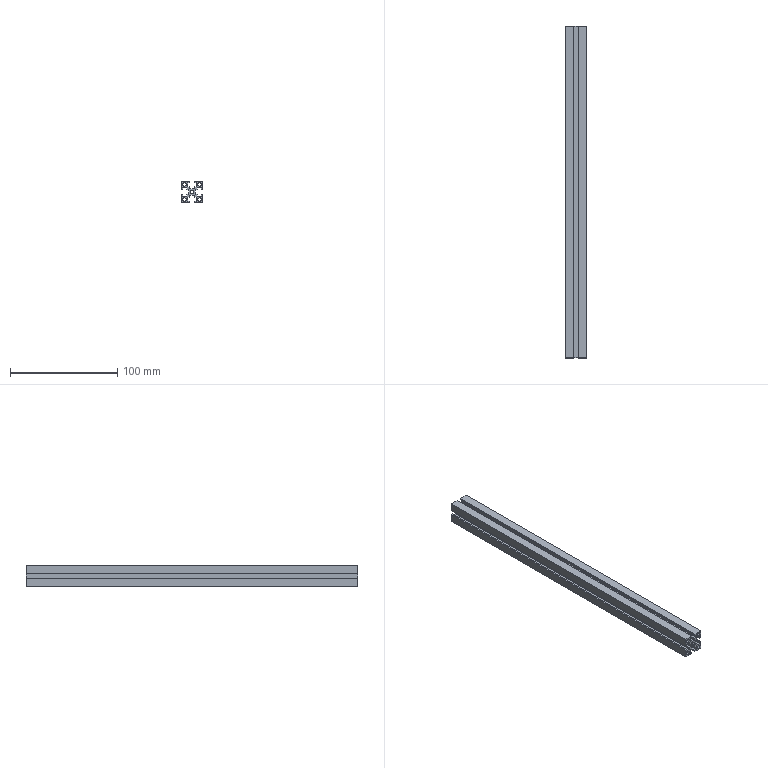Part | STEP file | 20 aluminium profile longitudinal 4 | 1 solid | 64 faces | box 20 x 310 x 20 mm | volume 55112 mm3 | plane 54 | cylinder 10 | commonest cylinder face diameters 3.3 x10